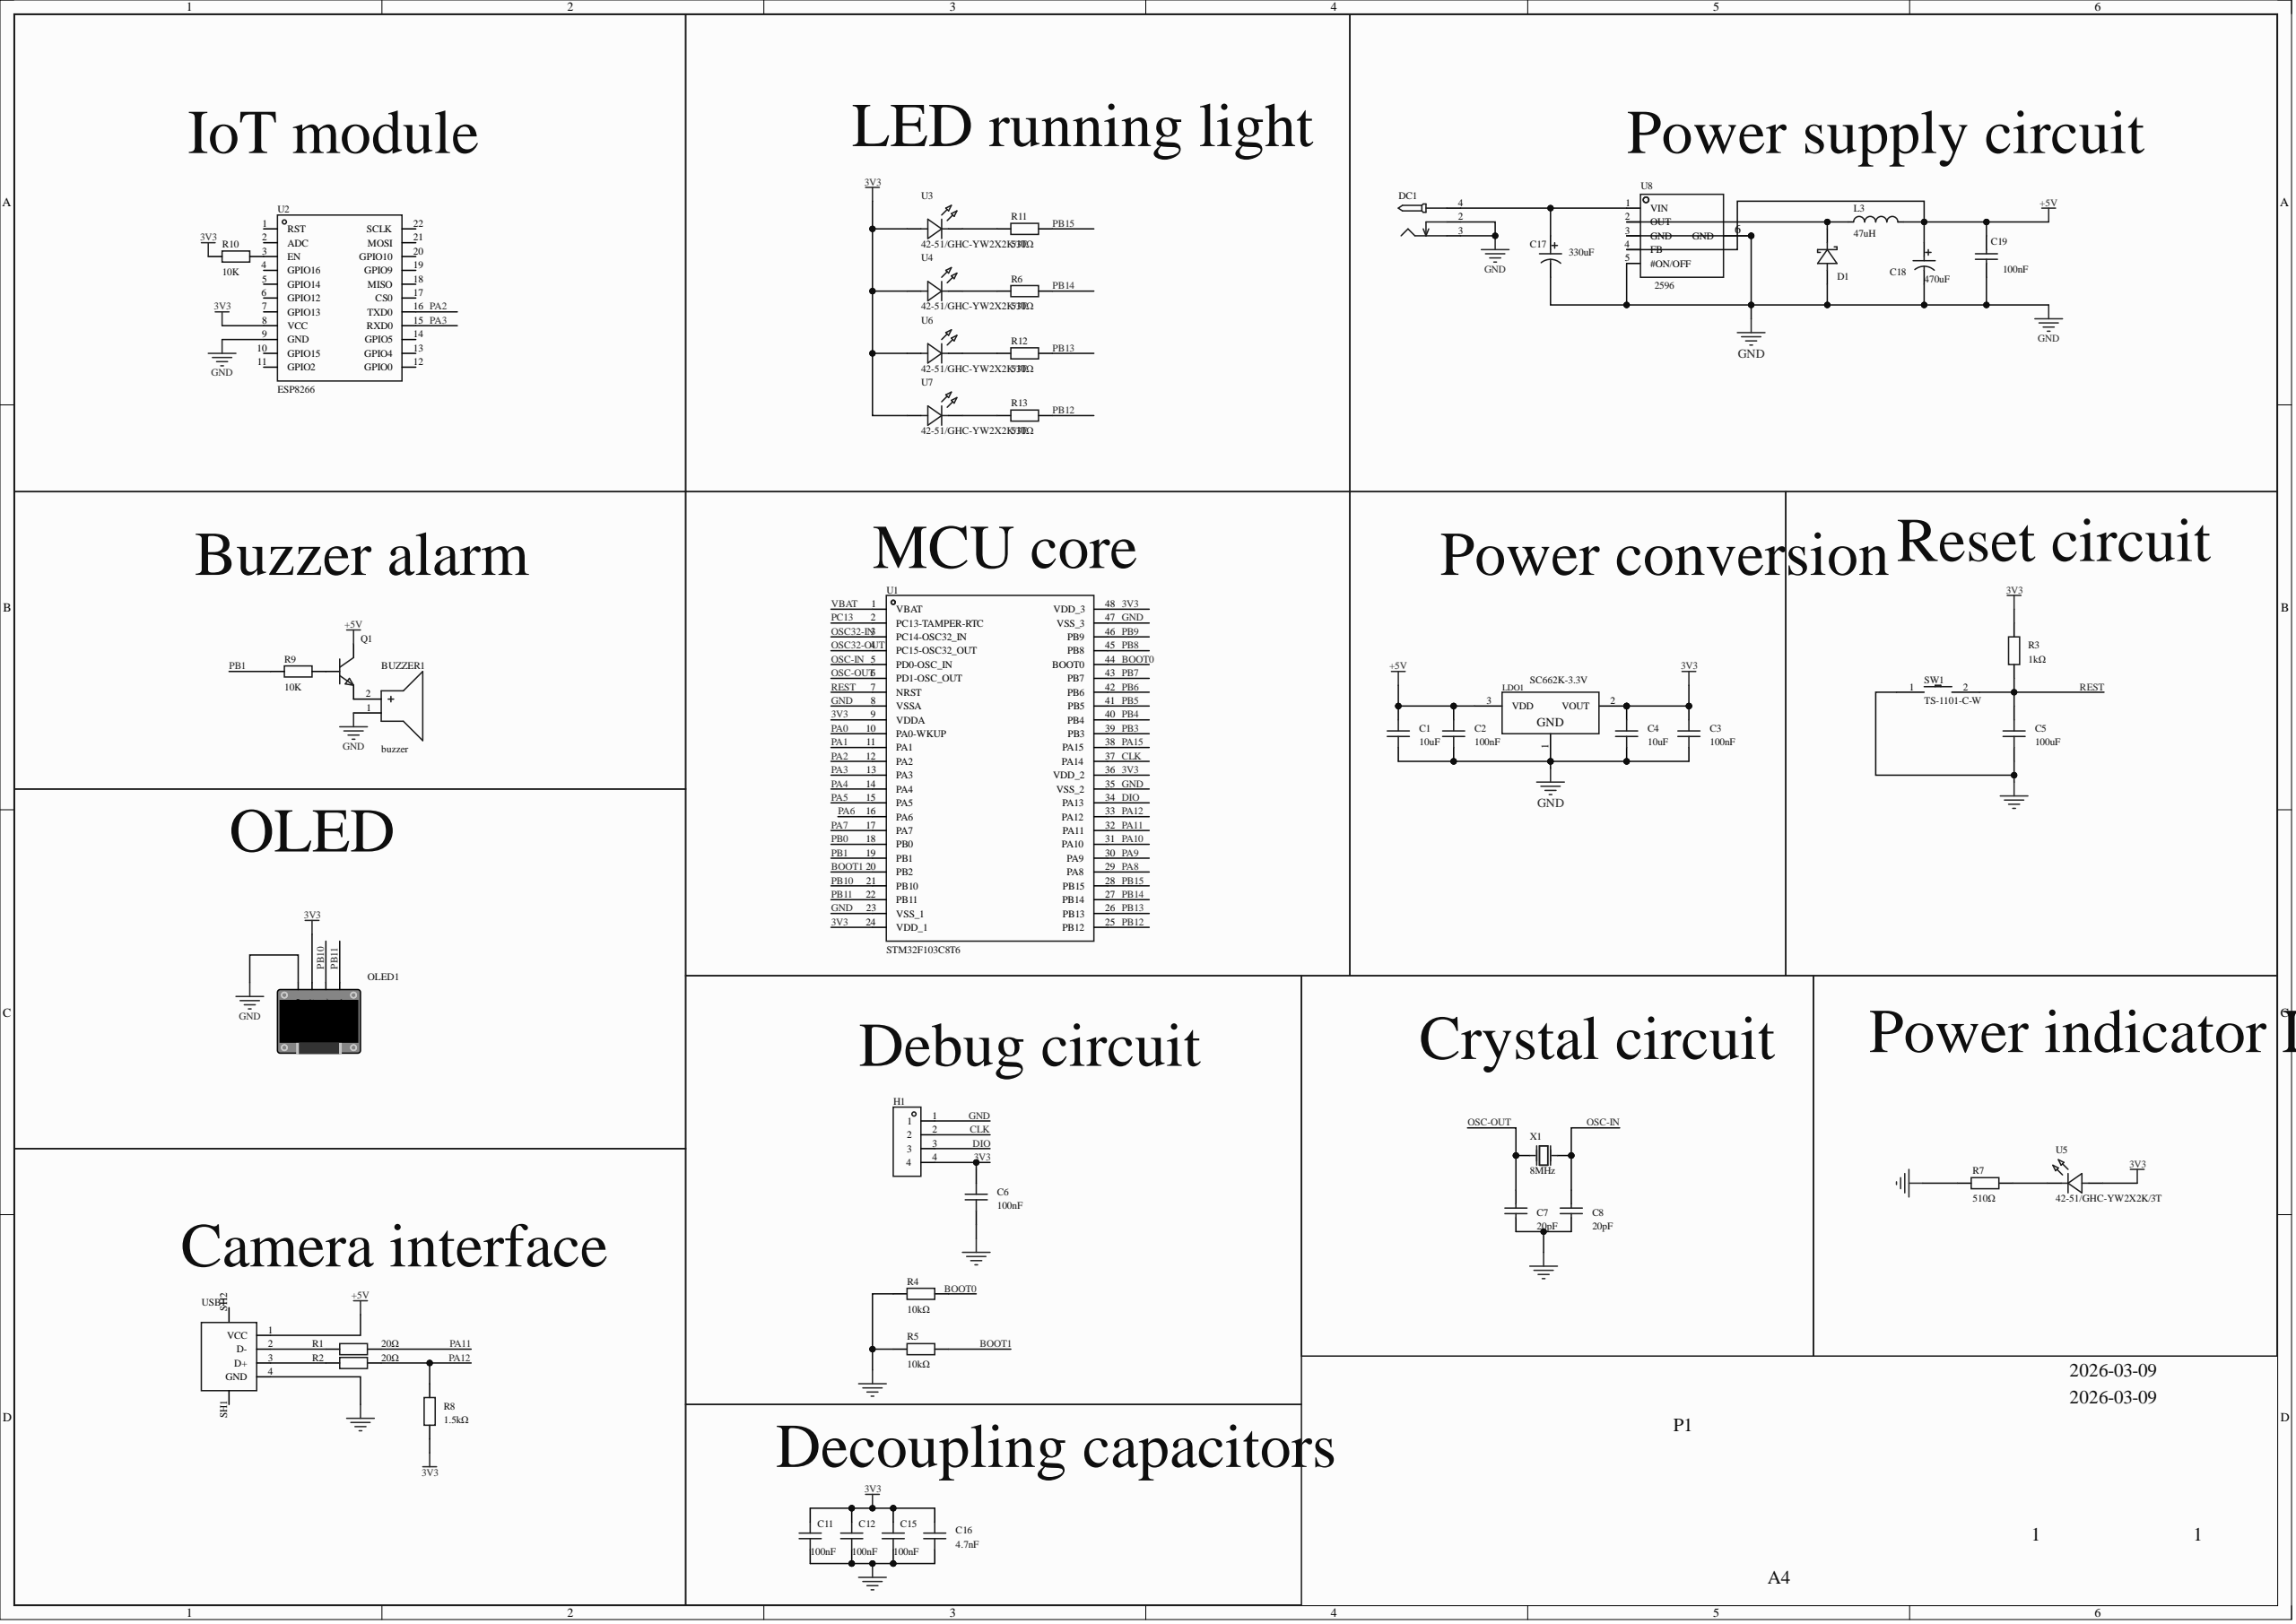Circuit board | Altium Designer | 47 parts | 33 nets
Bill of materials:
Comment,Description,Designator,Footprint,LibRef,Quantity
"buzzer","","BUZZER1","BUZ-TH_BD12.0-P6.00-D0.9-RD","buzzer","1"
"10uF","Capacitance: 10uF; tolerance: ±10%; rated voltage: 10V; dielectric (temperature coefficient): X5R;","C1, C4","C0603","CL10A106KP8NNNC","2"
"100nF","Capacitance: 100nF; tolerance: ±10%; rated voltage: 50V; dielectric (temperature coefficient): X7R;","C2, C3, C6, C11, C12, C15","C0603","CC0603KRX7R9BB104, CGA0603X7R104K500JT","6"
"100uF","Capacitance: 100uF; tolerance: ±20%; rated voltage: 10V; dielectric (temperature coefficient): X5R;","C5","C1206","HGC1206R5107M100NSPJ","1"
"20pF","Capacitance: 20pF; tolerance: ±5%; rated voltage: 50V; dielectric (temperature coefficient): C0G;","C7, C8","C0603","CL10C200JB8NNNC","2"
"4.7nF","Capacitance: 4.7nF; tolerance: ±10%; rated voltage: 50V; dielectric (temperature coefficient): X7R;","C16","C0603","CGA0603X7R472K500JT","1"
"","Capacitance: 220uF; tolerance: ±20%; rated voltage: 35V; can diameter: 8mm; can length: 10.5mm; ripple current: -; ESR: -; operating life: 2000hrs@105; operating temperature: -40~+105;","C17, C18","CAP-SMD_BD8.0-L8.3-W8.3-RD","CS1V221M-CRF10","2"
"","Capacitance: 100nF; tolerance: ±10%; rated voltage: 50V; temperature coefficient: X7R;","C19","C0805","CL21B104KBCNNNC","1"
"","","D1","SMA_L4.3-W2.6-LS5.2-RD","SS34_3","1"
"","","DC1","DC-2.0","DC-005_2.0","1"
"","","H1","HDR-TH_4P-P2.54-V-M","HDR-M_2.54_1x4P","1"
"","Inductance: 33uH; tolerance: ±20%; DC resistance (DCR): 270mΩ;","L3","IND-SMD_L7.0-W6.6","CMLO0630H330MTT","1"
"SC662K-3.3V","Output type: fixed; output polarity: positive; max input voltage: 6V; output voltage: 3.3V; output current: 250mA; power supply rejection ratio (PSRR): 50dB@(1kHz);","LDO1","SOT-23-3_L2.9-W1.3-P1.90-LS2.4-BR","SC662K-3.3V","1"
"","","OLED1","0.96OLED_4P","0.96OLED模块_4P","1"
"","","Q1","S8050_SOT-23","S8050_SOT_NPN","1"
"20Ω","Resistor type: thick film resistor; resistance: 20Ω; tolerance: ±1%; power: 100mW; max working voltage: 75V; temperature coefficient: ±100ppm/?;","R1, R2","R0603","0603WAF200JT5E","2"
"1kΩ","Resistor type: thick film resistor; resistance: 1kΩ; tolerance: ±1%; power: 100mW; max working voltage: 75V; temperature coefficient: ±100ppm/?;","R3","R0603","RC0603FR-071KL","1"
"10kΩ","Resistor type: thick film resistor; resistance: 10kΩ; tolerance: ±1%; power: 100mW; max working voltage: 75V; temperature coefficient: ±100ppm/?;","R4, R5","R0603","0603WAF1002T5E","2"
"510Ω","Resistor type: thick film resistor; resistance: 510Ω; tolerance: ±1%; power: 100mW; max working voltage: 75V; temperature coefficient: ±100ppm/?;","R6, R7, R11, R12, R13","R0603","0603WAF5100T5E","5"
"1.5kΩ","Resistor type: thick film resistor; resistance: 1.5kΩ; tolerance: ±1%; power: 100mW; max working voltage: 75V; temperature coefficient: ±100ppm/?;","R8","R0603","0603WAF1501T5E","1"
"10K","","R9, R10","R0603","Res_0603","2"
"TS-1101-C-W","Circuit structure: SPST; button shape: rectangular button; actuation force: 260gf; mounting: upright SMT; switch length: 6mm; switch width: 3.6mm; switch height: 2.5mm; with bracket: no; contact current: 50mA; rated voltage (AC): -; rated voltage (DC): 12V; rated power: -; insulation resistance: -; with lamp: no; mechanical life: 5 ten-thousand cycles;","SW1","SW-SMD_L6.0-W3.3-LS8.0","TS-1101-C-W","1"
"STM32F103C8T6","CPU core: ARM-M3; program memory capacity: 64KB; RAM total capacity: 20KB; GPIO port count: 37; operating voltage range: 2V~3.6V; max CPU frequency: 72MHz; program memory type: FLASH;","U1","LQFP-48_L7.0-W7.0-P0.50-LS9.0-BL","STM32F103C8T6","1"
"ESP8266","","U2","WIFIM-SMD_ESP-12F-ESP8266MOD","ESP8266","1"
"42-51/GHC-YW2X2K/3T","Emitted color: emerald green; forward current: -; dominant wavelength: 520nm~535nm; luminous intensity: 2850mcd;","U3, U4, U5, U6, U7","LED-SMD_L1.6-W0.8-FD_GREEN-1","42-51/GHC-YW2X2K/3T","5"
"LM2596S-5.0","Function type: step-down; output type: fixed; input voltage: 40V; output voltage: 5V; max output current: 3A;","U8","TO-263-5_L10.2-W8.9-P1.70-BR","LM2596S-5.0_C347421","1"
"","","USB1","USB_ Type-A","USB_ Type-A","1"
"8MHz","Crystal type: through-hole crystal; frequency: 8MHz; room-temperature frequency deviation: ±20ppm; load capacitance: 20pF; frequency stability (full temperature): ±30ppm;","X1","OSC-TH_L10.0-W4.5-P5.00","X49SD8MSD2SC","1"
Netlist (Protel format):
[
BUZZER1
BUZ-TH_BD12.0-P6.00-D0.9-RD
buzzer



]
[
C1
C0603
10uF



]
[
C2
C0603
100nF



]
[
C3
C0603
100nF



]
[
C4
C0603
10uF



]
[
C5
C1206
100uF



]
[
C6
C0603
100nF



]
[
C7
C0603
20pF



]
[
C8
C0603
20pF



]
[
C11
C0603
100nF



]
[
C12
C0603
100nF



]
[
C15
C0603
100nF



]
[
C16
C0603
4.7nF



]
[
C17
CAP-SMD_BD8.0-L8.3-W8.3-RD




]
[
C18
CAP-SMD_BD8.0-L8.3-W8.3-RD




]
[
C19
C0805




]
[
D1
SMA_L4.3-W2.6-LS5.2-RD




]
[
DC1
DC-2.0




]
[
H1
HDR-TH_4P-P2.54-V-M




]
[
L3
IND-SMD_L7.0-W6.6




]
[
LDO1
SOT-23-3_L2.9-W1.3-P1.90-LS2.4-BR
SC662K-3.3V



]
[
OLED1
0.96OLED_4P




]
[
Q1
S8050_SOT-23




]
[
R1
R0603
20Ω



]
[
R2
R0603
20Ω



]
[
R3
R0603
1kΩ



]
[
R4
R0603
10kΩ



]
[
R5
R0603
10kΩ



]
[
R6
R0603
510Ω



]
[
R7
R0603
510Ω



]
[
R8
R0603
1.5kΩ



]
[
R9
R0603
10K



]
[
R10
R0603
10K



]
[
R11
R0603
510Ω



]
[
R12
R0603
510Ω



]
[
R13
R0603
510Ω



]
[
SW1
SW-SMD_L6.0-W3.3-LS8.0
TS-1101-C-W



]
[
U1
LQFP-48_L7.0-W7.0-P0.50-LS9.0-BL
STM32F103C8T6



]
[
U2
WIFIM-SMD_ESP-12F-ESP8266MOD
ESP8266



]
[
U3
LED-SMD_L1.6-W0.8-FD_GREEN-1
42-51/GHC-YW2X2K/3T



]
[
U4
LED-SMD_L1.6-W0.8-FD_GREEN-1
42-51/GHC-YW2X2K/3T



]
[
U5
LED-SMD_L1.6-W0.8-FD_GREEN-1
42-51/GHC-YW2X2K/3T



]
[
U6
LED-SMD_L1.6-W0.8-FD_GREEN-1
42-51/GHC-YW2X2K/3T



]
[
U7
LED-SMD_L1.6-W0.8-FD_GREEN-1
42-51/GHC-YW2X2K/3T



]
[
U8
TO-263-5_L10.2-W8.9-P1.70-BR
LM2596S-5.0



]
[
USB1
USB_ Type-A




]
[
X1
OSC-TH_L10.0-W4.5-P5.00
8MHz



]
(
REST
C5-2
R3-1
SW1-2
U1-7
)
(
PB15
R11-2
U1-28
)
(
PB14
R6-2
U1-27
)
(
PB13
R12-2
U1-26
)
(
PB12
R13-2
U1-25
)
(
PB11
OLED1-4
U1-22
)
(
PB10
OLED1-3
U1-21
)
(
PB1
R9-1
U1-19
)
(
PA12
R2-2
R8-2
U1-33
)
(
PA11
R1-2
U1-32
)
(
PA3
U1-13
U2-15
)
(
PA2
U1-12
U2-16
)
(
OSC-OUT
C7-2
U1-6
X1-2
)
(
OSC-IN
C8-2
U1-5
X1-1
)
(
NetR13_1
R13-1
U7-2
)
(
NetR12_1
R12-1
U6-2
)
(
NetR11_1
R11-1
U3-2
)
(
NetR10_2
R10-2
U2-3
)
(
NetR7_1
R7-1
U5-2
)
(
NetR6_1
R6-1
U4-2
)
(
NetR2_1
R2-1
USB1-3
)
(
NetR1_1
R1-1
USB1-2
)
(
NetQ1_1
Q1-1
R9-2
)
(
NetD1_1
D1-1
L3-1
U8-2
)
(
NetC17_1
C17-1
DC1-4
U8-1
)
(
NetBUZZER1_2
BUZZER1-2
Q1-2
)
(
GND
BUZZER1-1
C1-1
C2-1
C3-1
C4-1
C5-1
C6-1
C7-1
C8-1
C11-1
C12-1
C15-1
C16-1
C17-2
C18-2
C19-2
D1-2
DC1-2
DC1-3
H1-1
LDO1-1
OLED1-1
R4-1
R5-1
R7-2
SW1-1
U1-8
U1-23
U1-35
U1-47
U2-9
U8-3
U8-5
U8-6
USB1-4
)
(
DIO
H1-3
U1-34
)
(
CLK
H1-2
U1-37
)
(
BOOT1
R5-2
U1-20
)
(
BOOT0
R4-2
U1-44
)
(
+5V
C1-2
C2-2
C18-1
C19-1
L3-2
LDO1-3
Q1-3
U8-4
USB1-1
)
(
3V3
C3-2
C4-2
C6-2
C11-2
C12-2
C15-2
C16-2
H1-4
LDO1-2
OLED1-2
R3-2
R8-1
R10-1
U1-9
U1-24
U1-36
U1-48
U2-8
U3-1
U4-1
U5-1
U6-1
U7-1
)